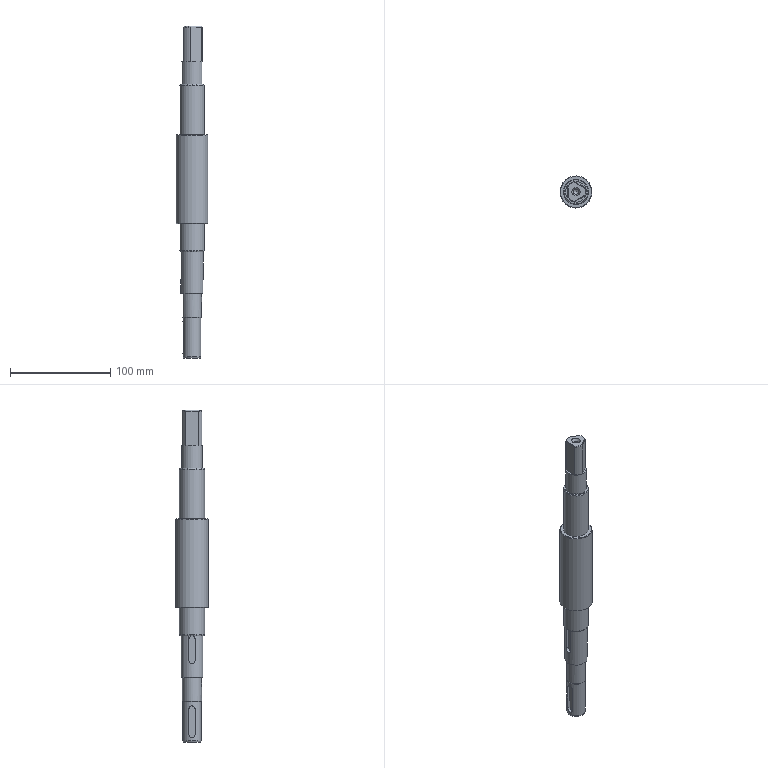CAM job | NX | 3+2 milling, drilling | part box 32 x 32 x 331.3 mm
Tools:
number,name,description,diameter,corner_radius,flute_length,length,flutes
1,ZXZ,Milling Tool-5 Parameters,6.0,0.0,50.0,75.0,2
15,5.0ZT,Drilling Tool,5.0,0.0,35.0,50.0,2
14,M6,Milling Tool-5 Parameters,5.0,0.0,30.0,30.0,4
12,D12,Milling Tool-5 Parameters,12.0,0.0,50.0,75.0,2
7,D6A45,Milling Tool-5 Parameters,6.0,0.0,50.0,75.0,2
4,D4,Milling Tool-5 Parameters,4.0,0.0,50.0,75.0,2
Operations:
program,operation,operation_type,tool,method,geometry_group,spindle_rpm,surface_speed,feed_per_tooth,feed_cut,feed_plunge,cut_length_mm,path_length_mm,cut_time_min,machine_time_min
1,DRILLING,Operation,ZXZ,METHOD,A,5000.0,94.0,0.025,250.0,0.0,4.0,68.0,0.016,0.0224
1,DRILLING_COPY_COPY_1,Operation,5.0ZT,METHOD,A,2000.0,56.0,0.0375,150.0,0.0,27.502,115.004,0.1833,0.1921
1,DRILLING_COPY_2_COPY_COPY_1_COPY_COPY,Operation,M6,METHOD,A,200.0,3.0,0.0013,1.0,0.0,26.0,112.0,26.0,26.009
1,ZLEVEL_PROFILE,ZLevelMilling,D12,METHOD,A,3000.0,94.0,0.3667,2200.0,1000.0,17339.153,17427.953,7.948,7.957
1,PLANAR_MILL_COPY_COPY,PlanarMilling,D6A45,METHOD,A,7500.0,141.0,0.0833,1250.0,100.0,32.307,91.307,0.0258,0.0317
1,PLANAR_MILL_COPY_COPY_COPY,PlanarMilling,D6A45,METHOD,A,7500.0,141.0,0.0833,1250.0,100.0,71.253,128.253,0.057,0.0627
1,刀补12,ZLevelMilling,D12,METHOD,A,5000.0,157.0,0.125,1250.0,100.0,3809.635,7169.204,3.048,3.384
2,刀补6,ZLevelMilling,D4,METHOD,B,6685.0,84.0,0.1234,1650.0,1000.0,2924.521,2994.96,1.781,1.788
2,刀补6_COPY,ZLevelMilling,D4,METHOD,B,6685.0,84.0,0.1234,1650.0,1000.0,2692.916,2768.3,1.64,1.648
3,刀补6_COPY_1,ZLevelMilling,D4,METHOD,C,6685.0,84.0,0.1234,1650.0,1000.0,1367.52,1438.567,0.837,0.8441